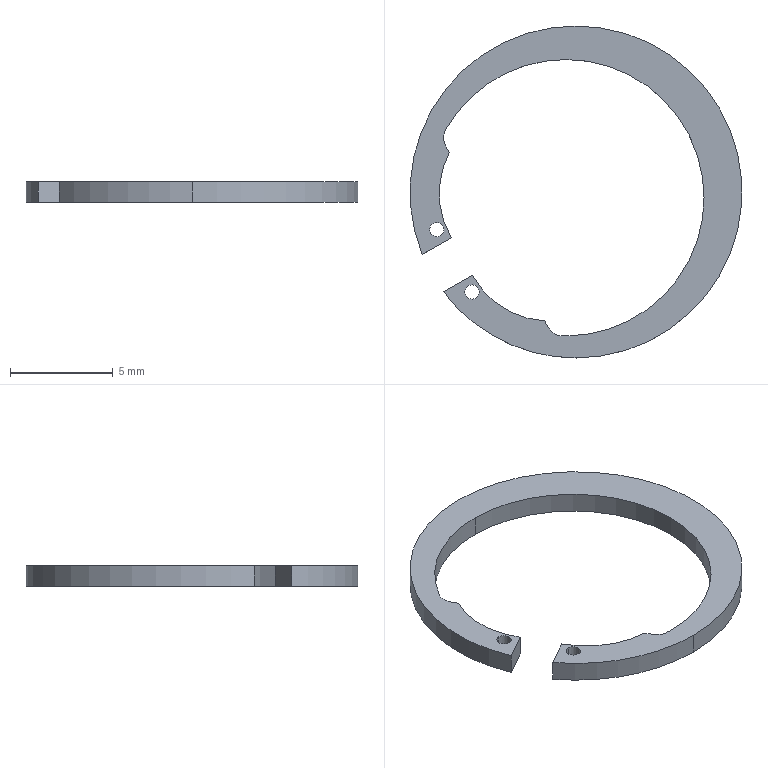Part | SolidWorks | features BaseBody 1 | 1 solid | 20 faces | box 16.193 x 16.193 x 1 mm | volume 66.891 mm3 | cylinder 14 | plane 6 | commonest cylinder face diameters 0.7 x4 13.482 x3 16.193 x3 1.613 x2 8.542 x2
STEP:
#1=CARTESIAN_POINT('',(553.328,-179.139,297.433));
#2=VERTEX_POINT('',#1);
#3=CARTESIAN_POINT('',(553.328,-178.439,297.433));
#4=VERTEX_POINT('',#3);
#5=CARTESIAN_POINT('',(553.328,-178.789,297.433));
#6=DIRECTION('',(-0.000000001,0.000000003,-1.));
#7=DIRECTION('',(0.,1.,0.000000003));
#8=AXIS2_PLACEMENT_3D('',#5,#6,#7);
#9=CIRCLE('',#8,0.35);
#10=EDGE_CURVE('',#2,#4,#9,.T.);
#11=ORIENTED_EDGE('',*,*,#10,.F.);
#12=CARTESIAN_POINT('',(553.328,-179.139,296.433));
#13=VERTEX_POINT('',#12);
#14=CARTESIAN_POINT('',(553.328,-179.139,296.433));
#15=DIRECTION('',(-0.000000001,0.000000003,-1.));
#16=VECTOR('',#15,1000.);
#17=LINE('',#14,#16);
#18=EDGE_CURVE('',#2,#13,#17,.T.);
#19=ORIENTED_EDGE('',*,*,#18,.T.);
#20=CARTESIAN_POINT('',(553.328,-178.439,296.433));
#21=VERTEX_POINT('',#20);
#22=CARTESIAN_POINT('',(553.328,-178.789,296.433));
#23=DIRECTION('',(0.000000001,-0.000000003,1.));
#24=DIRECTION('',(0.,1.,0.000000003));
#25=AXIS2_PLACEMENT_3D('',#22,#23,#24);
#26=CIRCLE('',#25,0.35);
#27=EDGE_CURVE('',#21,#13,#26,.T.);
#28=ORIENTED_EDGE('',*,*,#27,.F.);
#29=CARTESIAN_POINT('',(553.328,-178.439,296.433));
#30=DIRECTION('',(-0.000000001,0.000000003,-1.));
#31=VECTOR('',#30,1000.);
#32=LINE('',#29,#31);
#33=EDGE_CURVE('',#4,#21,#32,.T.);
#34=ORIENTED_EDGE('',*,*,#33,.F.);
#35=EDGE_LOOP('',(#11,#19,#28,#34));
#36=FACE_OUTER_BOUND('',#35,.T.);
#37=CARTESIAN_POINT('',(553.328,-178.789,296.433));
#38=DIRECTION('',(-0.000000001,0.000000003,-1.));
#39=DIRECTION('',(0.,1.,0.000000003));
#40=AXIS2_PLACEMENT_3D('',#37,#38,#39);
#41=CYLINDRICAL_SURFACE('',#40,0.35);
#42=ADVANCED_FACE('',(#36),#41,.F.);
#43=CARTESIAN_POINT('',(551.605,-176.093,297.433));
#44=VERTEX_POINT('',#43);
#45=CARTESIAN_POINT('',(551.605,-175.393,297.433));
#46=VERTEX_POINT('',#45);
#47=CARTESIAN_POINT('',(551.605,-175.743,297.433));
#48=DIRECTION('',(-0.000000001,0.000000003,-1.));
#49=DIRECTION('',(0.,1.,0.000000003));
#50=AXIS2_PLACEMENT_3D('',#47,#48,#49);
#51=CIRCLE('',#50,0.35);
#52=EDGE_CURVE('',#44,#46,#51,.T.);
#53=ORIENTED_EDGE('',*,*,#52,.F.);
#54=CARTESIAN_POINT('',(551.605,-176.093,296.433));
#55=VERTEX_POINT('',#54);
#56=CARTESIAN_POINT('',(551.605,-176.093,296.433));
#57=DIRECTION('',(-0.000000001,0.000000003,-1.));
#58=VECTOR('',#57,1000.);
#59=LINE('',#56,#58);
#60=EDGE_CURVE('',#44,#55,#59,.T.);
#61=ORIENTED_EDGE('',*,*,#60,.T.);
#62=CARTESIAN_POINT('',(551.605,-175.393,296.433));
#63=VERTEX_POINT('',#62);
#64=CARTESIAN_POINT('',(551.605,-175.743,296.433));
#65=DIRECTION('',(0.000000001,-0.000000003,1.));
#66=DIRECTION('',(0.,1.,0.000000003));
#67=AXIS2_PLACEMENT_3D('',#64,#65,#66);
#68=CIRCLE('',#67,0.35);
#69=EDGE_CURVE('',#63,#55,#68,.T.);
#70=ORIENTED_EDGE('',*,*,#69,.F.);
#71=CARTESIAN_POINT('',(551.605,-175.393,296.433));
#72=DIRECTION('',(-0.000000001,0.000000003,-1.));
#73=VECTOR('',#72,1000.);
#74=LINE('',#71,#73);
#75=EDGE_CURVE('',#46,#63,#74,.T.);
#76=ORIENTED_EDGE('',*,*,#75,.F.);
#77=EDGE_LOOP('',(#53,#61,#70,#76));
#78=FACE_OUTER_BOUND('',#77,.T.);
#79=CARTESIAN_POINT('',(551.605,-175.743,296.433));
#80=DIRECTION('',(-0.000000001,0.000000003,-1.));
#81=DIRECTION('',(0.,1.,0.000000003));
#82=AXIS2_PLACEMENT_3D('',#79,#80,#81);
#83=CYLINDRICAL_SURFACE('',#82,0.35);
#84=ADVANCED_FACE('',(#78),#83,.F.);
#85=CARTESIAN_POINT('',(557.906,-167.449,296.433));
#86=VERTEX_POINT('',#85);
#87=CARTESIAN_POINT('',(552.038,-170.871,296.433));
#88=VERTEX_POINT('',#87);
#89=CARTESIAN_POINT('',(557.906,-174.19,296.433));
#90=DIRECTION('',(0.000000001,-0.000000003,1.));
#91=DIRECTION('',(0.,-1.,-0.000000003));
#92=AXIS2_PLACEMENT_3D('',#89,#90,#91);
#93=CIRCLE('',#92,6.741);
#94=EDGE_CURVE('',#86,#88,#93,.T.);
#95=ORIENTED_EDGE('',*,*,#94,.F.);
#96=CARTESIAN_POINT('',(557.906,-167.449,297.433));
#97=VERTEX_POINT('',#96);
#98=CARTESIAN_POINT('',(557.906,-167.449,296.433));
#99=DIRECTION('',(0.000000001,-0.000000003,1.));
#100=VECTOR('',#99,1000.);
#101=LINE('',#98,#100);
#102=EDGE_CURVE('',#86,#97,#101,.T.);
#103=ORIENTED_EDGE('',*,*,#102,.T.);
#104=CARTESIAN_POINT('',(552.038,-170.871,297.433));
#105=VERTEX_POINT('',#104);
#106=CARTESIAN_POINT('',(557.906,-174.19,297.433));
#107=DIRECTION('',(-0.000000001,0.000000003,-1.));
#108=DIRECTION('',(0.,-1.,-0.000000003));
#109=AXIS2_PLACEMENT_3D('',#106,#107,#108);
#110=CIRCLE('',#109,6.741);
#111=EDGE_CURVE('',#105,#97,#110,.T.);
#112=ORIENTED_EDGE('',*,*,#111,.F.);
#113=CARTESIAN_POINT('',(552.038,-170.871,296.433));
#114=DIRECTION('',(0.000000001,-0.000000003,1.));
#115=VECTOR('',#114,1000.);
#116=LINE('',#113,#115);
#117=EDGE_CURVE('',#88,#105,#116,.T.);
#118=ORIENTED_EDGE('',*,*,#117,.F.);
#119=EDGE_LOOP('',(#95,#103,#112,#118));
#120=FACE_OUTER_BOUND('',#119,.T.);
#121=CARTESIAN_POINT('',(557.906,-174.19,296.433));
#122=DIRECTION('',(0.000000001,-0.000000003,1.));
#123=DIRECTION('',(0.,-1.,-0.000000003));
#124=AXIS2_PLACEMENT_3D('',#121,#122,#123);
#125=CYLINDRICAL_SURFACE('',#124,6.741);
#126=ADVANCED_FACE('',(#120),#125,.F.);
#127=ORIENTED_EDGE('',*,*,#102,.F.);
#128=CARTESIAN_POINT('',(557.906,-180.931,296.433));
#129=VERTEX_POINT('',#128);
#130=CARTESIAN_POINT('',(557.906,-174.19,296.433));
#131=DIRECTION('',(0.000000001,-0.000000003,1.));
#132=DIRECTION('',(0.,-1.,-0.000000003));
#133=AXIS2_PLACEMENT_3D('',#130,#131,#132);
#134=CIRCLE('',#133,6.741);
#135=EDGE_CURVE('',#129,#86,#134,.T.);
#136=ORIENTED_EDGE('',*,*,#135,.F.);
#137=CARTESIAN_POINT('',(557.906,-180.931,297.433));
#138=VERTEX_POINT('',#137);
#139=CARTESIAN_POINT('',(557.906,-180.931,296.433));
#140=DIRECTION('',(0.000000001,-0.000000003,1.));
#141=VECTOR('',#140,1000.);
#142=LINE('',#139,#141);
#143=EDGE_CURVE('',#129,#138,#142,.T.);
#144=ORIENTED_EDGE('',*,*,#143,.T.);
#145=CARTESIAN_POINT('',(557.906,-174.19,297.433));
#146=DIRECTION('',(-0.000000001,0.000000003,-1.));
#147=DIRECTION('',(0.,-1.,-0.000000003));
#148=AXIS2_PLACEMENT_3D('',#145,#146,#147);
#149=CIRCLE('',#148,6.741);
#150=EDGE_CURVE('',#97,#138,#149,.T.);
#151=ORIENTED_EDGE('',*,*,#150,.F.);
#152=EDGE_LOOP('',(#127,#136,#144,#151));
#153=FACE_OUTER_BOUND('',#152,.T.);
#154=CARTESIAN_POINT('',(557.906,-174.19,296.433));
#155=DIRECTION('',(0.000000001,-0.000000003,1.));
#156=DIRECTION('',(0.,-1.,-0.000000003));
#157=AXIS2_PLACEMENT_3D('',#154,#155,#156);
#158=CYLINDRICAL_SURFACE('',#157,6.741);
#159=ADVANCED_FACE('',(#153),#158,.F.);
#160=CARTESIAN_POINT('',(558.401,-182.006,296.433));
#161=VERTEX_POINT('',#160);
#162=CARTESIAN_POINT('',(558.401,-165.813,296.433));
#163=VERTEX_POINT('',#162);
#164=CARTESIAN_POINT('',(558.401,-173.91,296.433));
#165=DIRECTION('',(0.000000001,-0.000000003,1.));
#166=DIRECTION('',(0.,-1.,-0.000000003));
#167=AXIS2_PLACEMENT_3D('',#164,#165,#166);
#168=CIRCLE('',#167,8.097);
#169=EDGE_CURVE('',#161,#163,#168,.T.);
#170=ORIENTED_EDGE('',*,*,#169,.T.);
#171=CARTESIAN_POINT('',(558.401,-165.813,297.433));
#172=VERTEX_POINT('',#171);
#173=CARTESIAN_POINT('',(558.401,-165.813,296.433));
#174=DIRECTION('',(0.000000001,-0.000000003,1.));
#175=VECTOR('',#174,1000.);
#176=LINE('',#173,#175);
#177=EDGE_CURVE('',#163,#172,#176,.T.);
#178=ORIENTED_EDGE('',*,*,#177,.T.);
#179=CARTESIAN_POINT('',(558.401,-182.006,297.433));
#180=VERTEX_POINT('',#179);
#181=CARTESIAN_POINT('',(558.401,-173.91,297.433));
#182=DIRECTION('',(0.000000001,-0.000000003,1.));
#183=DIRECTION('',(0.,-1.,-0.000000003));
#184=AXIS2_PLACEMENT_3D('',#181,#182,#183);
#185=CIRCLE('',#184,8.097);
#186=EDGE_CURVE('',#180,#172,#185,.T.);
#187=ORIENTED_EDGE('',*,*,#186,.F.);
#188=CARTESIAN_POINT('',(558.401,-182.006,296.433));
#189=DIRECTION('',(0.000000001,-0.000000003,1.));
#190=VECTOR('',#189,1000.);
#191=LINE('',#188,#190);
#192=EDGE_CURVE('',#161,#180,#191,.T.);
#193=ORIENTED_EDGE('',*,*,#192,.F.);
#194=EDGE_LOOP('',(#170,#178,#187,#193));
#195=FACE_OUTER_BOUND('',#194,.T.);
#196=CARTESIAN_POINT('',(558.401,-173.91,296.433));
#197=DIRECTION('',(0.000000001,-0.000000003,1.));
#198=DIRECTION('',(0.,-1.,-0.000000003));
#199=AXIS2_PLACEMENT_3D('',#196,#197,#198);
#200=CYLINDRICAL_SURFACE('',#199,8.097);
#201=ADVANCED_FACE('',(#195),#200,.T.);
#202=CARTESIAN_POINT('',(551.93,-178.776,296.433));
#203=VERTEX_POINT('',#202);
#204=CARTESIAN_POINT('',(558.401,-173.91,296.433));
#205=DIRECTION('',(0.000000001,-0.000000003,1.));
#206=DIRECTION('',(0.,-1.,-0.000000003));
#207=AXIS2_PLACEMENT_3D('',#204,#205,#206);
#208=CIRCLE('',#207,8.097);
#209=EDGE_CURVE('',#203,#161,#208,.T.);
#210=ORIENTED_EDGE('',*,*,#209,.T.);
#211=ORIENTED_EDGE('',*,*,#192,.T.);
#212=CARTESIAN_POINT('',(551.93,-178.776,297.433));
#213=VERTEX_POINT('',#212);
#214=CARTESIAN_POINT('',(558.401,-173.91,297.433));
#215=DIRECTION('',(0.000000001,-0.000000003,1.));
#216=DIRECTION('',(0.,-1.,-0.000000003));
#217=AXIS2_PLACEMENT_3D('',#214,#215,#216);
#218=CIRCLE('',#217,8.097);
#219=EDGE_CURVE('',#213,#180,#218,.T.);
#220=ORIENTED_EDGE('',*,*,#219,.F.);
#221=CARTESIAN_POINT('',(551.93,-178.776,296.433));
#222=DIRECTION('',(-0.000000001,0.000000003,-1.));
#223=VECTOR('',#222,1000.);
#224=LINE('',#221,#223);
#225=EDGE_CURVE('',#213,#203,#224,.T.);
#226=ORIENTED_EDGE('',*,*,#225,.T.);
#227=EDGE_LOOP('',(#210,#211,#220,#226));
#228=FACE_OUTER_BOUND('',#227,.T.);
#229=CARTESIAN_POINT('',(558.401,-173.91,296.433));
#230=DIRECTION('',(0.000000001,-0.000000003,1.));
#231=DIRECTION('',(0.,-1.,-0.000000003));
#232=AXIS2_PLACEMENT_3D('',#229,#230,#231);
#233=CYLINDRICAL_SURFACE('',#232,8.097);
#234=ADVANCED_FACE('',(#228),#233,.T.);
#235=CARTESIAN_POINT('',(553.328,-178.789,297.433));
#236=DIRECTION('',(-0.000000001,0.000000003,-1.));
#237=DIRECTION('',(0.,1.,0.000000003));
#238=AXIS2_PLACEMENT_3D('',#235,#236,#237);
#239=CIRCLE('',#238,0.35);
#240=EDGE_CURVE('',#4,#2,#239,.T.);
#241=ORIENTED_EDGE('',*,*,#240,.T.);
#242=ORIENTED_EDGE('',*,*,#10,.T.);
#243=EDGE_LOOP('',(#241,#242));
#244=FACE_BOUND('',#243,.T.);
#245=CARTESIAN_POINT('',(551.605,-175.743,297.433));
#246=DIRECTION('',(-0.000000001,0.000000003,-1.));
#247=DIRECTION('',(0.,1.,0.000000003));
#248=AXIS2_PLACEMENT_3D('',#245,#246,#247);
#249=CIRCLE('',#248,0.35);
#250=EDGE_CURVE('',#46,#44,#249,.T.);
#251=ORIENTED_EDGE('',*,*,#250,.T.);
#252=ORIENTED_EDGE('',*,*,#52,.T.);
#253=EDGE_LOOP('',(#251,#252));
#254=FACE_BOUND('',#253,.T.);
#255=CARTESIAN_POINT('',(557.046,-180.519,297.433));
#256=VERTEX_POINT('',#255);
#257=CARTESIAN_POINT('',(556.864,-180.198,297.433));
#258=VERTEX_POINT('',#257);
#259=CARTESIAN_POINT('',(557.046,-180.519,297.433));
#260=DIRECTION('',(-0.4923,0.8704,0.000000003));
#261=VECTOR('',#260,1000.);
#262=LINE('',#259,#261);
#263=EDGE_CURVE('',#256,#258,#262,.T.);
#264=ORIENTED_EDGE('',*,*,#263,.T.);
#265=CARTESIAN_POINT('',(553.348,-177.973,297.433));
#266=VERTEX_POINT('',#265);
#267=CARTESIAN_POINT('',(557.101,-175.934,297.433));
#268=DIRECTION('',(-0.000000001,0.000000003,-1.));
#269=DIRECTION('',(0.,-1.,-0.000000003));
#270=AXIS2_PLACEMENT_3D('',#267,#268,#269);
#271=CIRCLE('',#270,4.271);
#272=EDGE_CURVE('',#258,#266,#271,.T.);
#273=ORIENTED_EDGE('',*,*,#272,.T.);
#274=CARTESIAN_POINT('',(553.348,-177.973,297.433));
#275=DIRECTION('',(-0.8704,-0.4923,-0.000000001));
#276=VECTOR('',#275,1000.);
#277=LINE('',#274,#276);
#278=EDGE_CURVE('',#266,#213,#277,.T.);
#279=ORIENTED_EDGE('',*,*,#278,.T.);
#280=ORIENTED_EDGE('',*,*,#219,.T.);
#281=ORIENTED_EDGE('',*,*,#186,.T.);
#282=CARTESIAN_POINT('',(550.896,-176.948,297.433));
#283=VERTEX_POINT('',#282);
#284=CARTESIAN_POINT('',(558.401,-173.91,297.433));
#285=DIRECTION('',(0.000000001,-0.000000003,1.));
#286=DIRECTION('',(0.,-1.,-0.000000003));
#287=AXIS2_PLACEMENT_3D('',#284,#285,#286);
#288=CIRCLE('',#287,8.097);
#289=EDGE_CURVE('',#172,#283,#288,.T.);
#290=ORIENTED_EDGE('',*,*,#289,.T.);
#291=CARTESIAN_POINT('',(552.315,-176.145,297.433));
#292=VERTEX_POINT('',#291);
#293=CARTESIAN_POINT('',(550.896,-176.948,297.433));
#294=DIRECTION('',(0.8704,0.4923,0.000000001));
#295=VECTOR('',#294,1000.);
#296=LINE('',#293,#295);
#297=EDGE_CURVE('',#283,#292,#296,.T.);
#298=ORIENTED_EDGE('',*,*,#297,.T.);
#299=CARTESIAN_POINT('',(552.22,-171.986,297.433));
#300=VERTEX_POINT('',#299);
#301=CARTESIAN_POINT('',(555.996,-173.981,297.433));
#302=DIRECTION('',(-0.000000001,0.000000003,-1.));
#303=DIRECTION('',(0.,-1.,-0.000000003));
#304=AXIS2_PLACEMENT_3D('',#301,#302,#303);
#305=CIRCLE('',#304,4.271);
#306=EDGE_CURVE('',#292,#300,#305,.T.);
#307=ORIENTED_EDGE('',*,*,#306,.T.);
#308=CARTESIAN_POINT('',(552.038,-171.665,297.433));
#309=VERTEX_POINT('',#308);
#310=CARTESIAN_POINT('',(552.22,-171.986,297.433));
#311=DIRECTION('',(-0.4923,0.8704,0.000000003));
#312=VECTOR('',#311,1000.);
#313=LINE('',#310,#312);
#314=EDGE_CURVE('',#300,#309,#313,.T.);
#315=ORIENTED_EDGE('',*,*,#314,.T.);
#316=CARTESIAN_POINT('',(552.74,-171.268,297.433));
#317=DIRECTION('',(-0.000000001,0.000000003,-1.));
#318=DIRECTION('',(0.,-1.,-0.000000003));
#319=AXIS2_PLACEMENT_3D('',#316,#317,#318);
#320=CIRCLE('',#319,0.8063);
#321=EDGE_CURVE('',#309,#105,#320,.T.);
#322=ORIENTED_EDGE('',*,*,#321,.T.);
#323=ORIENTED_EDGE('',*,*,#111,.T.);
#324=ORIENTED_EDGE('',*,*,#150,.T.);
#325=CARTESIAN_POINT('',(557.726,-180.928,297.433));
#326=VERTEX_POINT('',#325);
#327=CARTESIAN_POINT('',(557.906,-174.19,297.433));
#328=DIRECTION('',(-0.000000001,0.000000003,-1.));
#329=DIRECTION('',(0.,-1.,-0.000000003));
#330=AXIS2_PLACEMENT_3D('',#327,#328,#329);
#331=CIRCLE('',#330,6.741);
#332=EDGE_CURVE('',#138,#326,#331,.T.);
#333=ORIENTED_EDGE('',*,*,#332,.T.);
#334=CARTESIAN_POINT('',(557.748,-180.122,297.433));
#335=DIRECTION('',(-0.000000001,0.000000003,-1.));
#336=DIRECTION('',(0.,-1.,-0.000000003));
#337=AXIS2_PLACEMENT_3D('',#334,#335,#336);
#338=CIRCLE('',#337,0.8063);
#339=EDGE_CURVE('',#326,#256,#338,.T.);
#340=ORIENTED_EDGE('',*,*,#339,.T.);
#341=EDGE_LOOP('',(#264,#273,#279,#280,#281,#290,#298,#307,#315,#322,#323,#324,#333,#340));
#342=FACE_OUTER_BOUND('',#341,.T.);
#343=CARTESIAN_POINT('',(557.59,-174.37,297.433));
#344=DIRECTION('',(0.000000001,-0.000000003,1.));
#345=DIRECTION('',(0.,-1.,-0.000000003));
#346=AXIS2_PLACEMENT_3D('',#343,#344,#345);
#347=PLANE('',#346);
#348=ADVANCED_FACE('',(#244,#254,#342),#347,.T.);
#349=ORIENTED_EDGE('',*,*,#18,.F.);
#350=ORIENTED_EDGE('',*,*,#240,.F.);
#351=ORIENTED_EDGE('',*,*,#33,.T.);
#352=CARTESIAN_POINT('',(553.328,-178.789,296.433));
#353=DIRECTION('',(0.000000001,-0.000000003,1.));
#354=DIRECTION('',(0.,1.,0.000000003));
#355=AXIS2_PLACEMENT_3D('',#352,#353,#354);
#356=CIRCLE('',#355,0.35);
#357=EDGE_CURVE('',#13,#21,#356,.T.);
#358=ORIENTED_EDGE('',*,*,#357,.F.);
#359=EDGE_LOOP('',(#349,#350,#351,#358));
#360=FACE_OUTER_BOUND('',#359,.T.);
#361=CARTESIAN_POINT('',(553.328,-178.789,296.433));
#362=DIRECTION('',(-0.000000001,0.000000003,-1.));
#363=DIRECTION('',(0.,1.,0.000000003));
#364=AXIS2_PLACEMENT_3D('',#361,#362,#363);
#365=CYLINDRICAL_SURFACE('',#364,0.35);
#366=ADVANCED_FACE('',(#360),#365,.F.);
#367=ORIENTED_EDGE('',*,*,#60,.F.);
#368=ORIENTED_EDGE('',*,*,#250,.F.);
#369=ORIENTED_EDGE('',*,*,#75,.T.);
#370=CARTESIAN_POINT('',(551.605,-175.743,296.433));
#371=DIRECTION('',(0.000000001,-0.000000003,1.));
#372=DIRECTION('',(0.,1.,0.000000003));
#373=AXIS2_PLACEMENT_3D('',#370,#371,#372);
#374=CIRCLE('',#373,0.35);
#375=EDGE_CURVE('',#55,#63,#374,.T.);
#376=ORIENTED_EDGE('',*,*,#375,.F.);
#377=EDGE_LOOP('',(#367,#368,#369,#376));
#378=FACE_OUTER_BOUND('',#377,.T.);
#379=CARTESIAN_POINT('',(551.605,-175.743,296.433));
#380=DIRECTION('',(-0.000000001,0.000000003,-1.));
#381=DIRECTION('',(0.,1.,0.000000003));
#382=AXIS2_PLACEMENT_3D('',#379,#380,#381);
#383=CYLINDRICAL_SURFACE('',#382,0.35);
#384=ADVANCED_FACE('',(#378),#383,.F.);
#385=CARTESIAN_POINT('',(556.864,-180.198,296.433));
#386=VERTEX_POINT('',#385);
#387=CARTESIAN_POINT('',(556.864,-180.198,296.433));
#388=DIRECTION('',(0.000000001,-0.000000003,1.));
#389=VECTOR('',#388,1000.);
#390=LINE('',#387,#389);
#391=EDGE_CURVE('',#386,#258,#390,.T.);
#392=ORIENTED_EDGE('',*,*,#391,.F.);
#393=CARTESIAN_POINT('',(553.348,-177.973,296.433));
#394=VERTEX_POINT('',#393);
#395=CARTESIAN_POINT('',(557.101,-175.934,296.433));
#396=DIRECTION('',(0.000000001,-0.000000003,1.));
#397=DIRECTION('',(0.,-1.,-0.000000003));
#398=AXIS2_PLACEMENT_3D('',#395,#396,#397);
#399=CIRCLE('',#398,4.271);
#400=EDGE_CURVE('',#394,#386,#399,.T.);
#401=ORIENTED_EDGE('',*,*,#400,.F.);
#402=CARTESIAN_POINT('',(553.348,-177.973,296.433));
#403=DIRECTION('',(-0.000000001,0.000000003,-1.));
#404=VECTOR('',#403,1000.);
#405=LINE('',#402,#404);
#406=EDGE_CURVE('',#266,#394,#405,.T.);
#407=ORIENTED_EDGE('',*,*,#406,.F.);
#408=ORIENTED_EDGE('',*,*,#272,.F.);
#409=EDGE_LOOP('',(#392,#401,#407,#408));
#410=FACE_OUTER_BOUND('',#409,.T.);
#411=CARTESIAN_POINT('',(557.101,-175.934,296.433));
#412=DIRECTION('',(0.000000001,-0.000000003,1.));
#413=DIRECTION('',(0.,-1.,-0.000000003));
#414=AXIS2_PLACEMENT_3D('',#411,#412,#413);
#415=CYLINDRICAL_SURFACE('',#414,4.271);
#416=ADVANCED_FACE('',(#410),#415,.F.);
#417=CARTESIAN_POINT('',(557.046,-180.519,296.433));
#418=VERTEX_POINT('',#417);
#419=CARTESIAN_POINT('',(556.864,-180.198,296.433));
#420=DIRECTION('',(-0.4923,0.8704,0.));
#421=VECTOR('',#420,1000.);
#422=LINE('',#419,#421);
#423=EDGE_CURVE('',#418,#386,#422,.T.);
#424=ORIENTED_EDGE('',*,*,#423,.T.);
#425=ORIENTED_EDGE('',*,*,#391,.T.);
#426=ORIENTED_EDGE('',*,*,#263,.F.);
#427=CARTESIAN_POINT('',(557.046,-180.519,296.433));
#428=DIRECTION('',(0.000000001,0.,-1.));
#429=VECTOR('',#428,1000.);
#430=LINE('',#427,#429);
#431=EDGE_CURVE('',#256,#418,#430,.T.);
#432=ORIENTED_EDGE('',*,*,#431,.T.);
#433=EDGE_LOOP('',(#424,#425,#426,#432));
#434=FACE_OUTER_BOUND('',#433,.T.);
#435=CARTESIAN_POINT('',(556.864,-180.198,296.433));
#436=DIRECTION('',(0.8704,0.4923,0.000000001));
#437=DIRECTION('',(-0.4923,0.8704,0.));
#438=AXIS2_PLACEMENT_3D('',#435,#436,#437);
#439=PLANE('',#438);
#440=ADVANCED_FACE('',(#434),#439,.T.);
#441=CARTESIAN_POINT('',(557.726,-180.928,296.433));
#442=VERTEX_POINT('',#441);
#443=CARTESIAN_POINT('',(557.726,-180.928,296.433));
#444=DIRECTION('',(0.000000001,-0.000000003,1.));
#445=VECTOR('',#444,1000.);
#446=LINE('',#443,#445);
#447=EDGE_CURVE('',#442,#326,#446,.T.);
#448=ORIENTED_EDGE('',*,*,#447,.F.);
#449=CARTESIAN_POINT('',(557.748,-180.122,296.433));
#450=DIRECTION('',(0.000000001,-0.000000003,1.));
#451=DIRECTION('',(0.,-1.,-0.000000003));
#452=AXIS2_PLACEMENT_3D('',#449,#450,#451);
#453=CIRCLE('',#452,0.8063);
#454=EDGE_CURVE('',#418,#442,#453,.T.);
#455=ORIENTED_EDGE('',*,*,#454,.F.);
#456=ORIENTED_EDGE('',*,*,#431,.F.);
#457=ORIENTED_EDGE('',*,*,#339,.F.);
#458=EDGE_LOOP('',(#448,#455,#456,#457));
#459=FACE_OUTER_BOUND('',#458,.T.);
#460=CARTESIAN_POINT('',(557.748,-180.122,296.433));
#461=DIRECTION('',(0.000000001,-0.000000003,1.));
#462=DIRECTION('',(0.,-1.,-0.000000003));
#463=AXIS2_PLACEMENT_3D('',#460,#461,#462);
#464=CYLINDRICAL_SURFACE('',#463,0.8063);
#465=ADVANCED_FACE('',(#459),#464,.F.);
#466=ORIENTED_EDGE('',*,*,#143,.F.);
#467=CARTESIAN_POINT('',(557.906,-174.19,296.433));
#468=DIRECTION('',(0.000000001,-0.000000003,1.));
#469=DIRECTION('',(0.,-1.,-0.000000003));
#470=AXIS2_PLACEMENT_3D('',#467,#468,#469);
#471=CIRCLE('',#470,6.741);
#472=EDGE_CURVE('',#442,#129,#471,.T.);
#473=ORIENTED_EDGE('',*,*,#472,.F.);
#474=ORIENTED_EDGE('',*,*,#447,.T.);
#475=ORIENTED_EDGE('',*,*,#332,.F.);
#476=EDGE_LOOP('',(#466,#473,#474,#475));
#477=FACE_OUTER_BOUND('',#476,.T.);
#478=CARTESIAN_POINT('',(557.906,-174.19,296.433));
#479=DIRECTION('',(0.000000001,-0.000000003,1.));
#480=DIRECTION('',(0.,-1.,-0.000000003));
#481=AXIS2_PLACEMENT_3D('',#478,#479,#480);
#482=CYLINDRICAL_SURFACE('',#481,6.741);
#483=ADVANCED_FACE('',(#477),#482,.F.);
#484=CARTESIAN_POINT('',(552.038,-171.665,296.433));
#485=VERTEX_POINT('',#484);
#486=CARTESIAN_POINT('',(552.038,-171.665,296.433));
#487=DIRECTION('',(0.000000001,-0.000000003,1.));
#488=VECTOR('',#487,1000.);
#489=LINE('',#486,#488);
#490=EDGE_CURVE('',#485,#309,#489,.T.);
#491=ORIENTED_EDGE('',*,*,#490,.F.);
#492=CARTESIAN_POINT('',(552.74,-171.268,296.433));
#493=DIRECTION('',(0.000000001,-0.000000003,1.));
#494=DIRECTION('',(0.,-1.,-0.000000003));
#495=AXIS2_PLACEMENT_3D('',#492,#493,#494);
#496=CIRCLE('',#495,0.8063);
#497=EDGE_CURVE('',#88,#485,#496,.T.);
#498=ORIENTED_EDGE('',*,*,#497,.F.);
#499=ORIENTED_EDGE('',*,*,#117,.T.);
#500=ORIENTED_EDGE('',*,*,#321,.F.);
#501=EDGE_LOOP('',(#491,#498,#499,#500));
#502=FACE_OUTER_BOUND('',#501,.T.);
#503=CARTESIAN_POINT('',(552.74,-171.268,296.433));
#504=DIRECTION('',(0.000000001,-0.000000003,1.));
#505=DIRECTION('',(0.,-1.,-0.000000003));
#506=AXIS2_PLACEMENT_3D('',#503,#504,#505);
#507=CYLINDRICAL_SURFACE('',#506,0.8063);
#508=ADVANCED_FACE('',(#502),#507,.F.);
#509=CARTESIAN_POINT('',(552.22,-171.986,296.433));
#510=VERTEX_POINT('',#509);
#511=CARTESIAN_POINT('',(552.038,-171.665,296.433));
#512=DIRECTION('',(-0.4923,0.8704,0.));
#513=VECTOR('',#512,1000.);
#514=LINE('',#511,#513);
#515=EDGE_CURVE('',#510,#485,#514,.T.);
#516=ORIENTED_EDGE('',*,*,#515,.T.);
#517=ORIENTED_EDGE('',*,*,#490,.T.);
#518=ORIENTED_EDGE('',*,*,#314,.F.);
#519=CARTESIAN_POINT('',(552.22,-171.986,296.433));
#520=DIRECTION('',(0.000000001,0.,-1.));
#521=VECTOR('',#520,1000.);
#522=LINE('',#519,#521);
#523=EDGE_CURVE('',#300,#510,#522,.T.);
#524=ORIENTED_EDGE('',*,*,#523,.T.);
#525=EDGE_LOOP('',(#516,#517,#518,#524));
#526=FACE_OUTER_BOUND('',#525,.T.);
#527=CARTESIAN_POINT('',(552.038,-171.665,296.433));
#528=DIRECTION('',(0.8704,0.4923,0.000000001));
#529=DIRECTION('',(-0.4923,0.8704,0.));
#530=AXIS2_PLACEMENT_3D('',#527,#528,#529);
#531=PLANE('',#530);
#532=ADVANCED_FACE('',(#526),#531,.T.);
#533=CARTESIAN_POINT('',(552.315,-176.145,296.433));
#534=VERTEX_POINT('',#533);
#535=CARTESIAN_POINT('',(552.315,-176.145,296.433));
#536=DIRECTION('',(0.000000001,-0.000000003,1.));
#537=VECTOR('',#536,1000.);
#538=LINE('',#535,#537);
#539=EDGE_CURVE('',#534,#292,#538,.T.);
#540=ORIENTED_EDGE('',*,*,#539,.F.);
#541=CARTESIAN_POINT('',(555.996,-173.981,296.433));
#542=DIRECTION('',(0.000000001,-0.000000003,1.));
#543=DIRECTION('',(0.,-1.,-0.000000003));
#544=AXIS2_PLACEMENT_3D('',#541,#542,#543);
#545=CIRCLE('',#544,4.271);
#546=EDGE_CURVE('',#510,#534,#545,.T.);
#547=ORIENTED_EDGE('',*,*,#546,.F.);
#548=ORIENTED_EDGE('',*,*,#523,.F.);
#549=ORIENTED_EDGE('',*,*,#306,.F.);
#550=EDGE_LOOP('',(#540,#547,#548,#549));
#551=FACE_OUTER_BOUND('',#550,.T.);
#552=CARTESIAN_POINT('',(555.996,-173.981,296.433));
#553=DIRECTION('',(0.000000001,-0.000000003,1.));
#554=DIRECTION('',(0.,-1.,-0.000000003));
#555=AXIS2_PLACEMENT_3D('',#552,#553,#554);
#556=CYLINDRICAL_SURFACE('',#555,4.271);
#557=ADVANCED_FACE('',(#551),#556,.F.);
#558=CARTESIAN_POINT('',(550.896,-176.948,296.433));
#559=VERTEX_POINT('',#558);
#560=CARTESIAN_POINT('',(552.315,-176.145,296.433));
#561=DIRECTION('',(0.8704,0.4923,0.));
#562=VECTOR('',#561,1000.);
#563=LINE('',#560,#562);
#564=EDGE_CURVE('',#559,#534,#563,.T.);
#565=ORIENTED_EDGE('',*,*,#564,.T.);
#566=ORIENTED_EDGE('',*,*,#539,.T.);
#567=ORIENTED_EDGE('',*,*,#297,.F.);
#568=CARTESIAN_POINT('',(550.896,-176.948,296.433));
#569=DIRECTION('',(-0.000000002,0.000000003,-1.));
#570=VECTOR('',#569,1000.);
#571=LINE('',#568,#570);
#572=EDGE_CURVE('',#283,#559,#571,.T.);
#573=ORIENTED_EDGE('',*,*,#572,.T.);
#574=EDGE_LOOP('',(#565,#566,#567,#573));
#575=FACE_OUTER_BOUND('',#574,.T.);
#576=CARTESIAN_POINT('',(552.315,-176.145,296.433));
#577=DIRECTION('',(0.4923,-0.8704,-0.000000003));
#578=DIRECTION('',(0.8704,0.4923,0.));
#579=AXIS2_PLACEMENT_3D('',#576,#577,#578);
#580=PLANE('',#579);
#581=ADVANCED_FACE('',(#575),#580,.T.);
#582=ORIENTED_EDGE('',*,*,#177,.F.);
#583=CARTESIAN_POINT('',(558.401,-173.91,296.433));
#584=DIRECTION('',(0.000000001,-0.000000003,1.));
#585=DIRECTION('',(0.,-1.,-0.000000003));
#586=AXIS2_PLACEMENT_3D('',#583,#584,#585);
#587=CIRCLE('',#586,8.097);
#588=EDGE_CURVE('',#163,#559,#587,.T.);
#589=ORIENTED_EDGE('',*,*,#588,.T.);
#590=ORIENTED_EDGE('',*,*,#572,.F.);
#591=ORIENTED_EDGE('',*,*,#289,.F.);
#592=EDGE_LOOP('',(#582,#589,#590,#591));
#593=FACE_OUTER_BOUND('',#592,.T.);
#594=CARTESIAN_POINT('',(558.401,-173.91,296.433));
#595=DIRECTION('',(0.000000001,-0.000000003,1.));
#596=DIRECTION('',(0.,-1.,-0.000000003));
#597=AXIS2_PLACEMENT_3D('',#594,#595,#596);
#598=CYLINDRICAL_SURFACE('',#597,8.097);
#599=ADVANCED_FACE('',(#593),#598,.T.);
#600=CARTESIAN_POINT('',(551.93,-178.776,296.433));
#601=DIRECTION('',(-0.8704,-0.4923,0.));
#602=VECTOR('',#601,1000.);
#603=LINE('',#600,#602);
#604=EDGE_CURVE('',#394,#203,#603,.T.);
#605=ORIENTED_EDGE('',*,*,#604,.T.);
#606=ORIENTED_EDGE('',*,*,#225,.F.);
#607=ORIENTED_EDGE('',*,*,#278,.F.);
#608=ORIENTED_EDGE('',*,*,#406,.T.);
#609=EDGE_LOOP('',(#605,#606,#607,#608));
#610=FACE_OUTER_BOUND('',#609,.T.);
#611=CARTESIAN_POINT('',(551.93,-178.776,296.433));
#612=DIRECTION('',(-0.4923,0.8704,0.000000003));
#613=DIRECTION('',(-0.8704,-0.4923,0.));
#614=AXIS2_PLACEMENT_3D('',#611,#612,#613);
#615=PLANE('',#614);
#616=ADVANCED_FACE('',(#610),#615,.T.);
#617=ORIENTED_EDGE('',*,*,#27,.T.);
#618=ORIENTED_EDGE('',*,*,#357,.T.);
#619=EDGE_LOOP('',(#617,#618));
#620=FACE_BOUND('',#619,.T.);
#621=ORIENTED_EDGE('',*,*,#69,.T.);
#622=ORIENTED_EDGE('',*,*,#375,.T.);
#623=EDGE_LOOP('',(#621,#622));
#624=FACE_BOUND('',#623,.T.);
#625=ORIENTED_EDGE('',*,*,#604,.F.);
#626=ORIENTED_EDGE('',*,*,#400,.T.);
#627=ORIENTED_EDGE('',*,*,#423,.F.);
#628=ORIENTED_EDGE('',*,*,#454,.T.);
#629=ORIENTED_EDGE('',*,*,#472,.T.);
#630=ORIENTED_EDGE('',*,*,#135,.T.);
#631=ORIENTED_EDGE('',*,*,#94,.T.);
#632=ORIENTED_EDGE('',*,*,#497,.T.);
#633=ORIENTED_EDGE('',*,*,#515,.F.);
#634=ORIENTED_EDGE('',*,*,#546,.T.);
#635=ORIENTED_EDGE('',*,*,#564,.F.);
#636=ORIENTED_EDGE('',*,*,#588,.F.);
#637=ORIENTED_EDGE('',*,*,#169,.F.);
#638=ORIENTED_EDGE('',*,*,#209,.F.);
#639=EDGE_LOOP('',(#625,#626,#627,#628,#629,#630,#631,#632,#633,#634,#635,#636,#637,#638));
#640=FACE_OUTER_BOUND('',#639,.T.);
#641=CARTESIAN_POINT('',(557.59,-174.37,296.433));
#642=DIRECTION('',(0.000000001,-0.000000003,1.));
#643=DIRECTION('',(0.,-1.,-0.000000003));
#644=AXIS2_PLACEMENT_3D('',#641,#642,#643);
#645=PLANE('',#644);
#646=ADVANCED_FACE('',(#620,#624,#640),#645,.F.);
#647=CLOSED_SHELL('',(#42,#84,#126,#159,#201,#234,#348,#366,#384,#416,#440,#465,#483,#508,#532,#557,#581,#599,#616,#646));
#648=MANIFOLD_SOLID_BREP('',#647);
#649=CARTESIAN_POINT('',(0.,0.,0.));
#650=DIRECTION('',(0.,0.,1.));
#651=DIRECTION('',(1.,0.,0.));
#652=AXIS2_PLACEMENT_3D('',#649,#650,#651);
#653=(LENGTH_UNIT()NAMED_UNIT(*)SI_UNIT(.MILLI.,.METRE.));
#654=UNCERTAINTY_MEASURE_WITH_UNIT(LENGTH_MEASURE(0.00001),#653,'','');
#655=(NAMED_UNIT(*)PLANE_ANGLE_UNIT()SI_UNIT($,.RADIAN.));
#656=(NAMED_UNIT(*)SI_UNIT($,.STERADIAN.)SOLID_ANGLE_UNIT());
#657=(GEOMETRIC_REPRESENTATION_CONTEXT(3)GLOBAL_UNCERTAINTY_ASSIGNED_CONTEXT((#654))GLOBAL_UNIT_ASSIGNED_CONTEXT((#653,#655,#656))REPRESENTATION_CONTEXT('',''));
#658=ADVANCED_BREP_SHAPE_REPRESENTATION('',(#648,#652),#657);